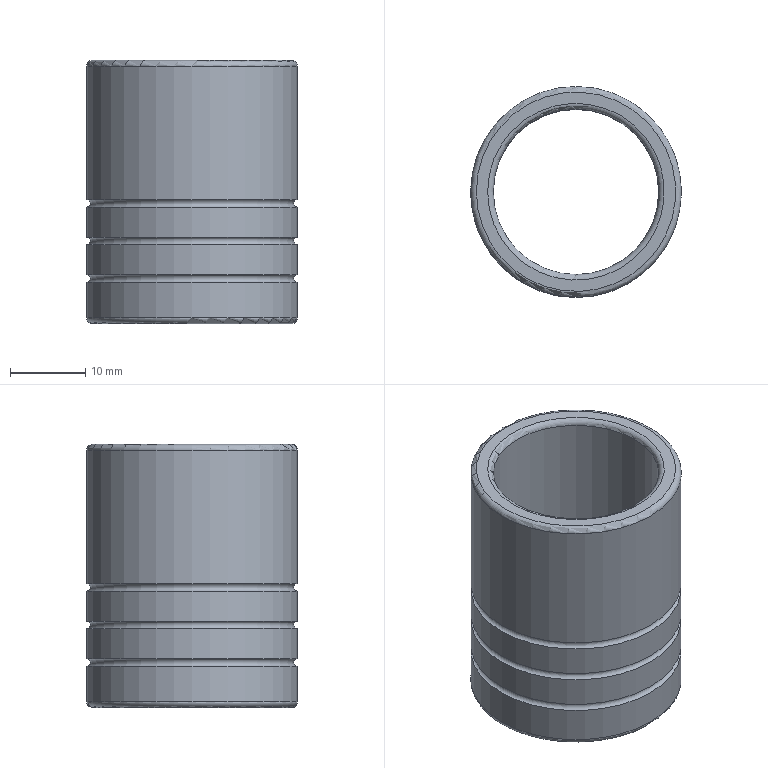Part | STEP file | 200 mesh_id1806 | 1 solid | 14 faces | box 28 x 28 x 35 mm | volume 8107 mm3 | torus 7 | cylinder 5 | plane 2 | commonest cylinder face diameters 28 x4 22 x1
STEP:
#1=CARTESIAN_POINT('',(-17063.884,-4095.269,38.75));
#2=VERTEX_POINT('',#1);
#3=CARTESIAN_POINT('',(-17052.884,-4095.269,38.75));
#4=DIRECTION('',(0.,0.,1.));
#5=DIRECTION('',(-1.,0.,0.));
#6=AXIS2_PLACEMENT_3D('',#3,#4,#5);
#7=CIRCLE('',#6,11.);
#8=EDGE_CURVE('',#2,#2,#7,.T.);
#9=ORIENTED_EDGE('',*,*,#8,.T.);
#10=EDGE_LOOP('',(#9));
#11=FACE_BOUND('',#10,.T.);
#12=CARTESIAN_POINT('',(-17041.884,-4095.269,5.25));
#13=VERTEX_POINT('',#12);
#14=CARTESIAN_POINT('',(-17052.884,-4095.269,5.25));
#15=DIRECTION('',(0.,0.,-1.));
#16=DIRECTION('',(1.,0.,0.));
#17=AXIS2_PLACEMENT_3D('',#14,#15,#16);
#18=CIRCLE('',#17,11.);
#19=EDGE_CURVE('',#13,#13,#18,.T.);
#20=ORIENTED_EDGE('',*,*,#19,.T.);
#21=EDGE_LOOP('',(#20));
#22=FACE_BOUND('',#21,.T.);
#23=CARTESIAN_POINT('',(-17052.884,-4095.269,49.5));
#24=DIRECTION('',(0.,0.,1.));
#25=DIRECTION('',(1.,0.,0.));
#26=AXIS2_PLACEMENT_3D('',#23,#24,#25);
#27=CYLINDRICAL_SURFACE('',#26,11.);
#28=ADVANCED_FACE('',(#11,#22),#27,.F.);
#29=CARTESIAN_POINT('',(-17039.634,-4095.269,4.5));
#30=VERTEX_POINT('',#29);
#31=CARTESIAN_POINT('',(-17052.884,-4095.269,4.5));
#32=DIRECTION('',(0.,0.,-1.));
#33=DIRECTION('',(1.,0.,0.));
#34=AXIS2_PLACEMENT_3D('',#31,#32,#33);
#35=CIRCLE('',#34,13.25);
#36=EDGE_CURVE('',#30,#30,#35,.T.);
#37=ORIENTED_EDGE('',*,*,#36,.T.);
#38=EDGE_LOOP('',(#37));
#39=FACE_BOUND('',#38,.T.);
#40=CARTESIAN_POINT('',(-17041.134,-4095.269,4.5));
#41=VERTEX_POINT('',#40);
#42=CARTESIAN_POINT('',(-17052.884,-4095.269,4.5));
#43=DIRECTION('',(0.,0.,1.));
#44=DIRECTION('',(1.,0.,0.));
#45=AXIS2_PLACEMENT_3D('',#42,#43,#44);
#46=CIRCLE('',#45,11.75);
#47=EDGE_CURVE('',#41,#41,#46,.T.);
#48=ORIENTED_EDGE('',*,*,#47,.T.);
#49=EDGE_LOOP('',(#48));
#50=FACE_BOUND('',#49,.T.);
#51=CARTESIAN_POINT('',(-17063.884,-4095.269,4.5));
#52=DIRECTION('',(0.,0.,1.));
#53=DIRECTION('',(1.,0.,0.));
#54=AXIS2_PLACEMENT_3D('',#51,#52,#53);
#55=PLANE('',#54);
#56=ADVANCED_FACE('',(#39,#50),#55,.F.);
#57=CARTESIAN_POINT('',(-17038.884,-4095.269,5.25));
#58=VERTEX_POINT('',#57);
#59=CARTESIAN_POINT('',(-17052.884,-4095.269,5.25));
#60=DIRECTION('',(0.,0.,1.));
#61=DIRECTION('',(1.,0.,0.));
#62=AXIS2_PLACEMENT_3D('',#59,#60,#61);
#63=CIRCLE('',#62,14.);
#64=EDGE_CURVE('',#58,#58,#63,.T.);
#65=ORIENTED_EDGE('',*,*,#64,.T.);
#66=EDGE_LOOP('',(#65));
#67=FACE_BOUND('',#66,.T.);
#68=CARTESIAN_POINT('',(-17038.884,-4095.269,10.));
#69=VERTEX_POINT('',#68);
#70=CARTESIAN_POINT('',(-17052.884,-4095.269,10.));
#71=DIRECTION('',(0.,0.,1.));
#72=DIRECTION('',(1.,0.,0.));
#73=AXIS2_PLACEMENT_3D('',#70,#71,#72);
#74=CIRCLE('',#73,14.);
#75=EDGE_CURVE('',#69,#69,#74,.T.);
#76=ORIENTED_EDGE('',*,*,#75,.F.);
#77=EDGE_LOOP('',(#76));
#78=FACE_BOUND('',#77,.T.);
#79=CARTESIAN_POINT('',(-17052.884,-4095.269,49.5));
#80=DIRECTION('',(0.,0.,1.));
#81=DIRECTION('',(1.,0.,0.));
#82=AXIS2_PLACEMENT_3D('',#79,#80,#81);
#83=CYLINDRICAL_SURFACE('',#82,14.);
#84=ADVANCED_FACE('',(#67,#78),#83,.T.);
#85=CARTESIAN_POINT('',(-17038.884,-4095.269,11.));
#86=VERTEX_POINT('',#85);
#87=CARTESIAN_POINT('',(-17052.884,-4095.269,11.));
#88=DIRECTION('',(0.,0.,1.));
#89=DIRECTION('',(1.,0.,0.));
#90=AXIS2_PLACEMENT_3D('',#87,#88,#89);
#91=CIRCLE('',#90,14.);
#92=EDGE_CURVE('',#86,#86,#91,.T.);
#93=ORIENTED_EDGE('',*,*,#92,.F.);
#94=EDGE_LOOP('',(#93));
#95=FACE_BOUND('',#94,.T.);
#96=ORIENTED_EDGE('',*,*,#75,.T.);
#97=EDGE_LOOP('',(#96));
#98=FACE_BOUND('',#97,.T.);
#99=CARTESIAN_POINT('',(-17052.884,-4095.269,10.5));
#100=DIRECTION('',(0.,0.,1.));
#101=DIRECTION('',(1.,0.,0.));
#102=AXIS2_PLACEMENT_3D('',#99,#100,#101);
#103=TOROIDAL_SURFACE('',#102,14.,0.5);
#104=ADVANCED_FACE('',(#95,#98),#103,.F.);
#105=CARTESIAN_POINT('',(-17038.884,-4095.269,15.));
#106=VERTEX_POINT('',#105);
#107=CARTESIAN_POINT('',(-17052.884,-4095.269,15.));
#108=DIRECTION('',(0.,0.,1.));
#109=DIRECTION('',(1.,0.,0.));
#110=AXIS2_PLACEMENT_3D('',#107,#108,#109);
#111=CIRCLE('',#110,14.);
#112=EDGE_CURVE('',#106,#106,#111,.T.);
#113=ORIENTED_EDGE('',*,*,#112,.F.);
#114=EDGE_LOOP('',(#113));
#115=FACE_BOUND('',#114,.T.);
#116=ORIENTED_EDGE('',*,*,#92,.T.);
#117=EDGE_LOOP('',(#116));
#118=FACE_BOUND('',#117,.T.);
#119=CARTESIAN_POINT('',(-17052.884,-4095.269,49.5));
#120=DIRECTION('',(0.,0.,1.));
#121=DIRECTION('',(1.,0.,0.));
#122=AXIS2_PLACEMENT_3D('',#119,#120,#121);
#123=CYLINDRICAL_SURFACE('',#122,14.);
#124=ADVANCED_FACE('',(#115,#118),#123,.T.);
#125=CARTESIAN_POINT('',(-17038.884,-4095.269,16.));
#126=VERTEX_POINT('',#125);
#127=CARTESIAN_POINT('',(-17052.884,-4095.269,16.));
#128=DIRECTION('',(0.,0.,1.));
#129=DIRECTION('',(1.,0.,0.));
#130=AXIS2_PLACEMENT_3D('',#127,#128,#129);
#131=CIRCLE('',#130,14.);
#132=EDGE_CURVE('',#126,#126,#131,.T.);
#133=ORIENTED_EDGE('',*,*,#132,.F.);
#134=EDGE_LOOP('',(#133));
#135=FACE_BOUND('',#134,.T.);
#136=ORIENTED_EDGE('',*,*,#112,.T.);
#137=EDGE_LOOP('',(#136));
#138=FACE_BOUND('',#137,.T.);
#139=CARTESIAN_POINT('',(-17052.884,-4095.269,15.5));
#140=DIRECTION('',(0.,0.,1.));
#141=DIRECTION('',(1.,0.,0.));
#142=AXIS2_PLACEMENT_3D('',#139,#140,#141);
#143=TOROIDAL_SURFACE('',#142,14.,0.5);
#144=ADVANCED_FACE('',(#135,#138),#143,.F.);
#145=CARTESIAN_POINT('',(-17038.884,-4095.269,20.));
#146=VERTEX_POINT('',#145);
#147=CARTESIAN_POINT('',(-17052.884,-4095.269,20.));
#148=DIRECTION('',(0.,0.,1.));
#149=DIRECTION('',(1.,0.,0.));
#150=AXIS2_PLACEMENT_3D('',#147,#148,#149);
#151=CIRCLE('',#150,14.);
#152=EDGE_CURVE('',#146,#146,#151,.T.);
#153=ORIENTED_EDGE('',*,*,#152,.F.);
#154=EDGE_LOOP('',(#153));
#155=FACE_BOUND('',#154,.T.);
#156=ORIENTED_EDGE('',*,*,#132,.T.);
#157=EDGE_LOOP('',(#156));
#158=FACE_BOUND('',#157,.T.);
#159=CARTESIAN_POINT('',(-17052.884,-4095.269,49.5));
#160=DIRECTION('',(0.,0.,1.));
#161=DIRECTION('',(1.,0.,0.));
#162=AXIS2_PLACEMENT_3D('',#159,#160,#161);
#163=CYLINDRICAL_SURFACE('',#162,14.);
#164=ADVANCED_FACE('',(#155,#158),#163,.T.);
#165=CARTESIAN_POINT('',(-17038.884,-4095.269,21.));
#166=VERTEX_POINT('',#165);
#167=CARTESIAN_POINT('',(-17052.884,-4095.269,21.));
#168=DIRECTION('',(0.,0.,1.));
#169=DIRECTION('',(1.,0.,0.));
#170=AXIS2_PLACEMENT_3D('',#167,#168,#169);
#171=CIRCLE('',#170,14.);
#172=EDGE_CURVE('',#166,#166,#171,.T.);
#173=ORIENTED_EDGE('',*,*,#172,.F.);
#174=EDGE_LOOP('',(#173));
#175=FACE_BOUND('',#174,.T.);
#176=ORIENTED_EDGE('',*,*,#152,.T.);
#177=EDGE_LOOP('',(#176));
#178=FACE_BOUND('',#177,.T.);
#179=CARTESIAN_POINT('',(-17052.884,-4095.269,20.5));
#180=DIRECTION('',(0.,0.,1.));
#181=DIRECTION('',(1.,0.,0.));
#182=AXIS2_PLACEMENT_3D('',#179,#180,#181);
#183=TOROIDAL_SURFACE('',#182,14.,0.5);
#184=ADVANCED_FACE('',(#175,#178),#183,.F.);
#185=CARTESIAN_POINT('',(-17066.884,-4095.269,38.75));
#186=VERTEX_POINT('',#185);
#187=CARTESIAN_POINT('',(-17052.884,-4095.269,38.75));
#188=DIRECTION('',(0.,0.,-1.));
#189=DIRECTION('',(-1.,0.,0.));
#190=AXIS2_PLACEMENT_3D('',#187,#188,#189);
#191=CIRCLE('',#190,14.);
#192=EDGE_CURVE('',#186,#186,#191,.T.);
#193=ORIENTED_EDGE('',*,*,#192,.T.);
#194=EDGE_LOOP('',(#193));
#195=FACE_BOUND('',#194,.T.);
#196=ORIENTED_EDGE('',*,*,#172,.T.);
#197=EDGE_LOOP('',(#196));
#198=FACE_BOUND('',#197,.T.);
#199=CARTESIAN_POINT('',(-17052.884,-4095.269,49.5));
#200=DIRECTION('',(0.,0.,1.));
#201=DIRECTION('',(1.,0.,0.));
#202=AXIS2_PLACEMENT_3D('',#199,#200,#201);
#203=CYLINDRICAL_SURFACE('',#202,14.);
#204=ADVANCED_FACE('',(#195,#198),#203,.T.);
#205=CARTESIAN_POINT('',(-17064.634,-4095.269,39.5));
#206=VERTEX_POINT('',#205);
#207=CARTESIAN_POINT('',(-17052.884,-4095.269,39.5));
#208=DIRECTION('',(0.,0.,-1.));
#209=DIRECTION('',(-1.,0.,0.));
#210=AXIS2_PLACEMENT_3D('',#207,#208,#209);
#211=CIRCLE('',#210,11.75);
#212=EDGE_CURVE('',#206,#206,#211,.T.);
#213=ORIENTED_EDGE('',*,*,#212,.T.);
#214=EDGE_LOOP('',(#213));
#215=FACE_BOUND('',#214,.T.);
#216=CARTESIAN_POINT('',(-17066.134,-4095.269,39.5));
#217=VERTEX_POINT('',#216);
#218=CARTESIAN_POINT('',(-17052.884,-4095.269,39.5));
#219=DIRECTION('',(0.,0.,1.));
#220=DIRECTION('',(-1.,0.,0.));
#221=AXIS2_PLACEMENT_3D('',#218,#219,#220);
#222=CIRCLE('',#221,13.25);
#223=EDGE_CURVE('',#217,#217,#222,.T.);
#224=ORIENTED_EDGE('',*,*,#223,.T.);
#225=EDGE_LOOP('',(#224));
#226=FACE_BOUND('',#225,.T.);
#227=CARTESIAN_POINT('',(-17066.884,-4095.269,39.5));
#228=DIRECTION('',(0.,0.,-1.));
#229=DIRECTION('',(-1.,0.,0.));
#230=AXIS2_PLACEMENT_3D('',#227,#228,#229);
#231=PLANE('',#230);
#232=ADVANCED_FACE('',(#215,#226),#231,.F.);
#233=ORIENTED_EDGE('',*,*,#36,.F.);
#234=EDGE_LOOP('',(#233));
#235=FACE_BOUND('',#234,.T.);
#236=ORIENTED_EDGE('',*,*,#64,.F.);
#237=EDGE_LOOP('',(#236));
#238=FACE_BOUND('',#237,.T.);
#239=CARTESIAN_POINT('',(-17052.884,-4095.269,5.25));
#240=DIRECTION('',(0.,0.,1.));
#241=DIRECTION('',(1.,0.,0.));
#242=AXIS2_PLACEMENT_3D('',#239,#240,#241);
#243=TOROIDAL_SURFACE('',#242,13.25,0.75);
#244=ADVANCED_FACE('',(#235,#238),#243,.T.);
#245=ORIENTED_EDGE('',*,*,#212,.F.);
#246=EDGE_LOOP('',(#245));
#247=FACE_BOUND('',#246,.T.);
#248=ORIENTED_EDGE('',*,*,#8,.F.);
#249=EDGE_LOOP('',(#248));
#250=FACE_BOUND('',#249,.T.);
#251=CARTESIAN_POINT('',(-17052.884,-4095.269,38.75));
#252=DIRECTION('',(0.,0.,-1.));
#253=DIRECTION('',(-1.,0.,0.));
#254=AXIS2_PLACEMENT_3D('',#251,#252,#253);
#255=TOROIDAL_SURFACE('',#254,11.75,0.75);
#256=ADVANCED_FACE('',(#247,#250),#255,.T.);
#257=ORIENTED_EDGE('',*,*,#192,.F.);
#258=EDGE_LOOP('',(#257));
#259=FACE_BOUND('',#258,.T.);
#260=ORIENTED_EDGE('',*,*,#223,.F.);
#261=EDGE_LOOP('',(#260));
#262=FACE_BOUND('',#261,.T.);
#263=CARTESIAN_POINT('',(-17052.884,-4095.269,38.75));
#264=DIRECTION('',(0.,0.,-1.));
#265=DIRECTION('',(-1.,0.,0.));
#266=AXIS2_PLACEMENT_3D('',#263,#264,#265);
#267=TOROIDAL_SURFACE('',#266,13.25,0.75);
#268=ADVANCED_FACE('',(#259,#262),#267,.T.);
#269=ORIENTED_EDGE('',*,*,#19,.F.);
#270=EDGE_LOOP('',(#269));
#271=FACE_BOUND('',#270,.T.);
#272=ORIENTED_EDGE('',*,*,#47,.F.);
#273=EDGE_LOOP('',(#272));
#274=FACE_BOUND('',#273,.T.);
#275=CARTESIAN_POINT('',(-17052.884,-4095.269,5.25));
#276=DIRECTION('',(0.,0.,1.));
#277=DIRECTION('',(1.,0.,0.));
#278=AXIS2_PLACEMENT_3D('',#275,#276,#277);
#279=TOROIDAL_SURFACE('',#278,11.75,0.75);
#280=ADVANCED_FACE('',(#271,#274),#279,.T.);
#281=CLOSED_SHELL('',(#28,#56,#84,#104,#124,#144,#164,#184,#204,#232,#244,#256,#268,#280));
#282=MANIFOLD_SOLID_BREP('',#281);
#283=(LENGTH_UNIT()NAMED_UNIT(*)SI_UNIT(.MILLI.,.METRE.));
#284=UNCERTAINTY_MEASURE_WITH_UNIT(LENGTH_MEASURE(0.00002),#283,'','');
#285=(NAMED_UNIT(*)PLANE_ANGLE_UNIT()SI_UNIT($,.RADIAN.));
#286=PLANE_ANGLE_MEASURE_WITH_UNIT(PLANE_ANGLE_MEASURE(0.01745),#285);
#287=DIMENSIONAL_EXPONENTS(0.,0.,0.,0.,0.,0.,0.);
#288=(CONVERSION_BASED_UNIT('DEGREE',#286)NAMED_UNIT(#287)PLANE_ANGLE_UNIT());
#289=(NAMED_UNIT(*)SI_UNIT($,.STERADIAN.)SOLID_ANGLE_UNIT());
#290=(GEOMETRIC_REPRESENTATION_CONTEXT(3)GLOBAL_UNCERTAINTY_ASSIGNED_CONTEXT((#284))GLOBAL_UNIT_ASSIGNED_CONTEXT((#283,#288,#289))REPRESENTATION_CONTEXT('',''));
#291=ADVANCED_BREP_SHAPE_REPRESENTATION('',(#282),#290);